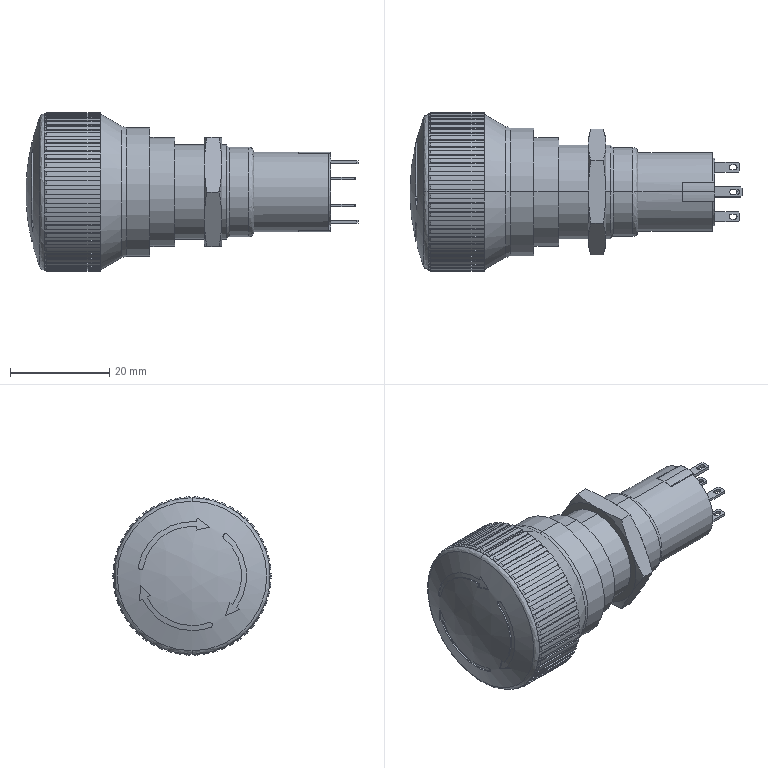Part | STEP file | LAS1_AGQ_TS[LAS1_AGQ_TS]_LAS1_AGQ_TS | 13 solids | 474 faces | box 67 x 32 x 31.988 mm | volume 25923 mm3 | plane 282 | cylinder 107 | cone 72 | spline 13 | commonest cylinder face diameters 32 x54 1 x24 22 x6 16 x5 19 x4 20 x4